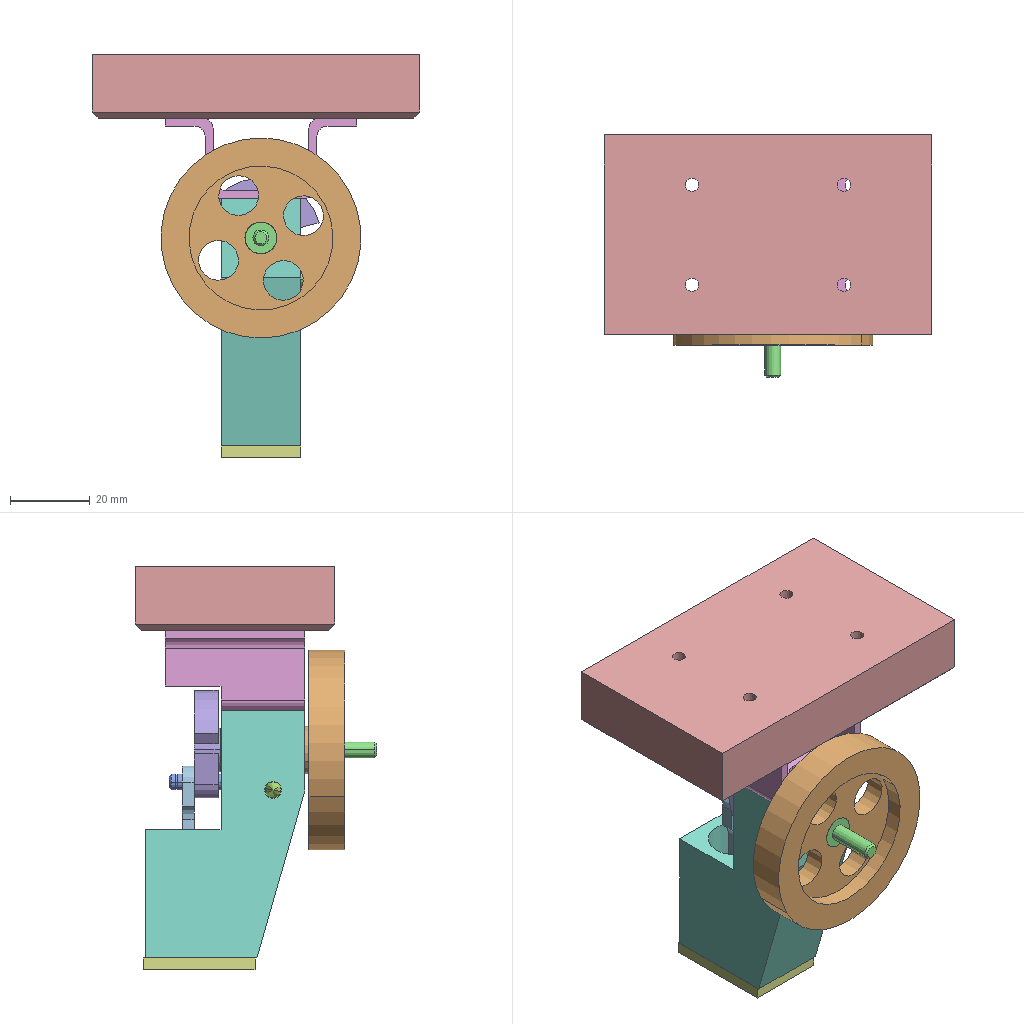Assembly | SolidWorks | 11 different items | 11 placed | box 82 x 61 x 101 mm
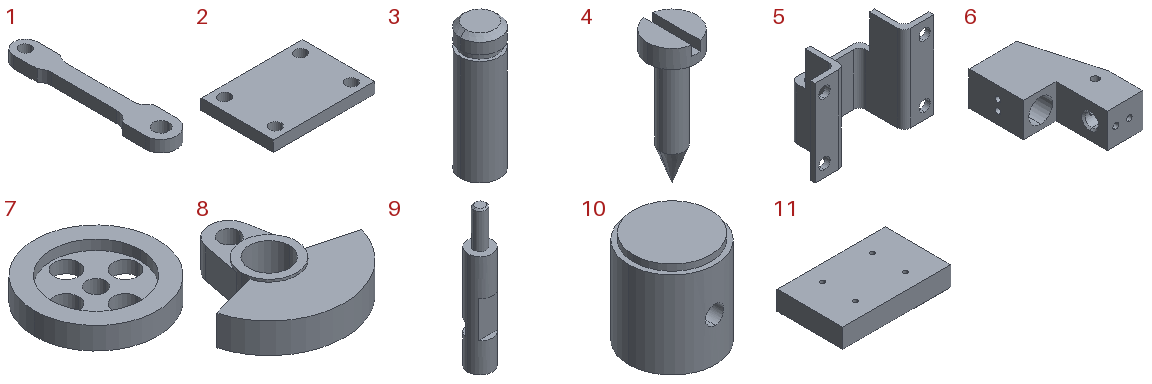Parts list (item | quantity | size | volume | features):
1 | x1 | 8 x 42 x 3 mm | 603.988 mm3 | features Extrusion 1
2 | x1 | 28 x 20 x 3 mm | 1583 mm3 | features Extrusion 1
3 | x1 | 4 x 4 x 13 mm | 159.831 mm3 | features ICE 2, Chamfer 1, Extrusion 1
4 | x1 | 8 x 8 x 22 mm | 325.653 mm3 | features ICE 2, Extrusion 1, RevCut 1
5 | x1 | 48 x 20 x 35 mm | 4681 mm3 | features ICE 2, Extrusion 1
6 | x1 | 40 x 62 x 20 mm | 25911 mm3 | features ICE 6, HoleWzd 4, 3DProfileFeature 3, Chamfer 2, Extrusion 1, LPattern 1, RefAxis 1
7 | x1 | 50 x 50 x 10 mm | 11841 mm3 | features ICE 4, Extrusion 1
8 | x1 | 28.914 x 27 x 6.5 mm | 2065 mm3 | features ICE 2, Extrusion 1
9 | x1 | 8 x 8 x 45.7 mm | 1609 mm3 | features ICE 4, 3DProfileFeature 2, HoleWzd 2, Chamfer 1, Extrusion 1, RefAxis 1
10 | x1 | 14 x 14 x 15 mm | 1304 mm3 | features ICE 3, 3DProfileFeature 1, Extrusion 1, HoleWzd 1
11 | x1 | 82 x 50 x 16 mm | 64760 mm3 | features 3DProfileFeature 1, Chamfer 1, Extrusion 1, HoleWzd 1, LPattern 1
Mates (type | each side: item.copy, entity, surface, feature):
Coincident | 11.1 plane | assembly plane | 3 times
Concentric | 11.1 face cylinder LPattern1 | 5.1 face cylinder Cut-Extrude2 | 2 times
Coincident | 11.1 face plane Boss-Extrude1 | 5.1 face plane Boss-Extrude1
Concentric | 5.1 face cylinder Cut-Extrude2 | 6.1 face cylinder M4 Tapped Hole2
Concentric | 5.1 face cylinder Cut-Extrude2 | 6.1 face cylinder M4 Tapped Hole3
Coincident | 5.1 face plane Boss-Extrude1 | 6.1 face plane Boss-Extrude1
Concentric | 6.1 face cylinder Cut-Extrude4 | 8.1 face cylinder Boss-Extrude2
Concentric | 6.1 face cylinder M3 Tapped Hole1 | 2.1 face cylinder Boss-Extrude1
Concentric | 6.1 face cylinder LPattern1 | 2.1 face cylinder Boss-Extrude1
Coincident | 6.1 face plane Boss-Extrude1 | 2.1 face plane Boss-Extrude1
Concentric | 6.1 face cylinder Cut-Extrude1 | 10.1 face cylinder Boss-Extrude1
Concentric | 4.1 face cylinder Boss-Extrude2 | 6.1 face cylinder M5 Tapped Hole1
Coincident | 8.1 face plane Boss-Extrude2 | 1.1 face plane Boss-Extrude1
Concentric | 3.1 face cylinder Boss-Extrude1 | 1.1 face cylinder Boss-Extrude1
Concentric | 3.1 face cylinder Boss-Extrude1 | 8.1 face cylinder Boss-Extrude3
Concentric | 3.1 face cylinder Boss-Extrude1 | assembly axis
Lock | 3.1 select_type:0 | assembly select_type:0
Concentric | 10.1 face cylinder Cut-Extrude3 | 1.1 face cylinder Boss-Extrude1
Concentric | 6.1 face cylinder Cut-Extrude4 | 7.1 face cylinder Cut-Extrude3
Coincident | 8.1 face plane Boss-Extrude2 | 9.1 face plane Boss-Extrude1
Concentric | 6.1 face cylinder Cut-Extrude5 | 9.1 face cylinder Ø3.2 (3.2) Diameter Hole2
Concentric | 6.1 select_type:25 | 9.1 face cylinder Boss-Extrude4
Coincident | 6.1 face plane Boss-Extrude1 | 7.1 face plane Boss-Extrude2
Concentric | 1.1 face cylinder Boss-Extrude1 | assembly face
Coincident | 1.1 face plane Boss-Extrude1 | assembly face
Concentric | 5.1 face cylinder Cut-Extrude2 | assembly face | 4 times
Coincident | 5.1 face plane Boss-Extrude1 | assembly face | 4 times
Concentric | 2.1 face cylinder Boss-Extrude1 | assembly face | 4 times
Coincident | 2.1 face plane Boss-Extrude1 | assembly face | 4 times
Concentric | 10.1 face cylinder Cut-Extrude3 | assembly face
Tangent | 10.1 face cylinder Boss-Extrude1 | assembly face
Coincident | 3.1 face plane Boss-Extrude1 | 6.1 face plane Boss-Extrude1